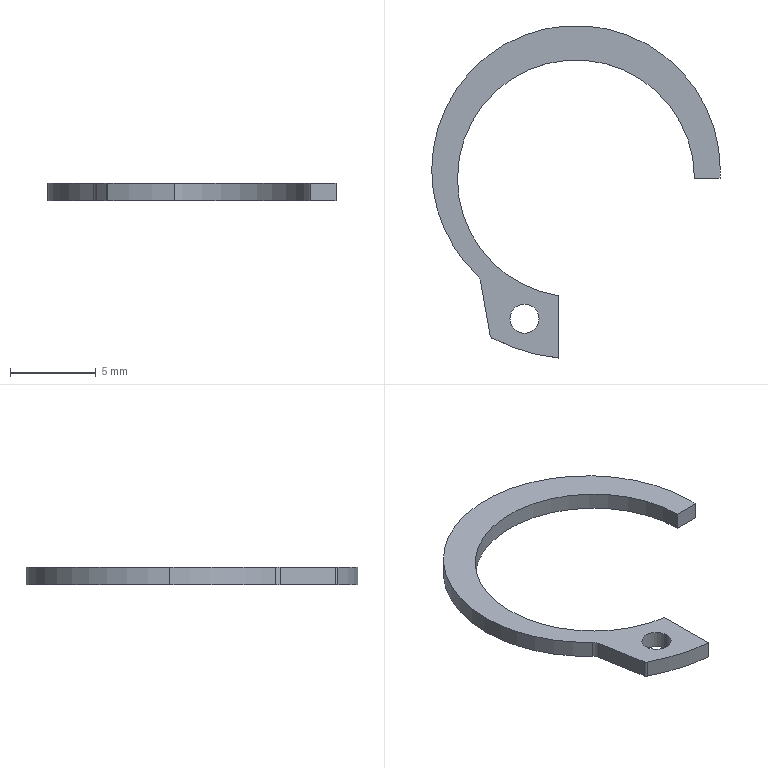Part | STEP file | Shaft retaining ring type A 15 | 1 solid | 15 faces | box 16.8 x 19.352 x 1 mm | volume 66.829 mm3 | cylinder 10 | plane 5 | commonest cylinder face diameters 16.8 x3 1.7 x2 13.8 x2 0.4 x1 1 x1 21 x1
STEP:
#1=CARTESIAN_POINT('',(0.,0.,0.));
#2=DIRECTION('',(0.,0.,1.));
#3=DIRECTION('',(1.,0.,0.));
#4=AXIS2_PLACEMENT_3D('',#1,#2,#3);
#5=CARTESIAN_POINT('',(-3.85,-8.666,0.5));
#6=VERTEX_POINT('',#5);
#7=CARTESIAN_POINT('',(-3.85,-8.666,-0.5));
#8=VERTEX_POINT('',#7);
#9=CARTESIAN_POINT('',(-3.85,-8.666,0.5));
#10=DIRECTION('',(0.,0.,-1.));
#11=VECTOR('',#10,1.);
#12=LINE('',#9,#11);
#13=CARTESIAN_POINT('',(-3.,-8.666,0.5));
#14=DIRECTION('',(0.,0.,-1.));
#15=DIRECTION('',(-1.,0.,0.));
#16=AXIS2_PLACEMENT_3D('',#13,#14,#15);
#17=CYLINDRICAL_SURFACE('',#16,0.85);
#18=CARTESIAN_POINT('',(6.283,0.));
#19=DIRECTION('',(0.,1.));
#20=VECTOR('',#19,1.);
#21=LINE('',#18,#20);
#22=(GEOMETRIC_REPRESENTATION_CONTEXT(2)PARAMETRIC_REPRESENTATION_CONTEXT()REPRESENTATION_CONTEXT('',''));
#23=DEFINITIONAL_REPRESENTATION('',(#21),#22);
#24=PCURVE('',#17,#23);
#25=CARTESIAN_POINT('',(-3.,-8.666,0.5));
#26=DIRECTION('',(0.,0.,-1.));
#27=DIRECTION('',(-1.,0.,0.));
#28=AXIS2_PLACEMENT_3D('',#25,#26,#27);
#29=CYLINDRICAL_SURFACE('',#28,0.85);
#30=CARTESIAN_POINT('',(0.,0.));
#31=DIRECTION('',(0.,1.));
#32=VECTOR('',#31,1.);
#33=LINE('',#30,#32);
#34=(GEOMETRIC_REPRESENTATION_CONTEXT(2)PARAMETRIC_REPRESENTATION_CONTEXT()REPRESENTATION_CONTEXT('',''));
#35=DEFINITIONAL_REPRESENTATION('',(#33),#34);
#36=PCURVE('',#29,#35);
#37=SURFACE_CURVE('',#12,(#24,#36),.PCURVE_S1.);
#38=EDGE_CURVE('',#6,#8,#37,.T.);
#39=ORIENTED_EDGE('',*,*,#38,.T.);
#40=CARTESIAN_POINT('',(-2.15,-8.666,-0.5));
#41=VERTEX_POINT('',#40);
#42=CARTESIAN_POINT('',(-3.,-8.666,-0.5));
#43=DIRECTION('',(0.,0.,1.));
#44=DIRECTION('',(1.,0.,0.));
#45=AXIS2_PLACEMENT_3D('',#42,#43,#44);
#46=CIRCLE('',#45,0.85);
#47=CARTESIAN_POINT('',(9.425,1.));
#48=DIRECTION('',(-1.,0.));
#49=VECTOR('',#48,1.);
#50=LINE('',#47,#49);
#51=(GEOMETRIC_REPRESENTATION_CONTEXT(2)PARAMETRIC_REPRESENTATION_CONTEXT()REPRESENTATION_CONTEXT('',''));
#52=DEFINITIONAL_REPRESENTATION('',(#50),#51);
#53=PCURVE('',#17,#52);
#54=CARTESIAN_POINT('',(-6.059,-6.519,-0.5));
#55=DIRECTION('',(0.,0.,1.));
#56=DIRECTION('',(1.,0.,0.));
#57=AXIS2_PLACEMENT_3D('',#54,#55,#56);
#58=PLANE('',#57);
#59=CARTESIAN_POINT('',(3.059,-2.147));
#60=DIRECTION('',(1.,0.));
#61=AXIS2_PLACEMENT_2D('',#59,#60);
#62=CIRCLE('',#61,0.85);
#63=(GEOMETRIC_REPRESENTATION_CONTEXT(2)PARAMETRIC_REPRESENTATION_CONTEXT()REPRESENTATION_CONTEXT('',''));
#64=DEFINITIONAL_REPRESENTATION('',(#62),#63);
#65=PCURVE('',#58,#64);
#66=SURFACE_CURVE('',#46,(#53,#65),.PCURVE_S1.);
#67=EDGE_CURVE('',#8,#41,#66,.T.);
#68=ORIENTED_EDGE('',*,*,#67,.T.);
#69=CARTESIAN_POINT('',(-2.15,-8.666,0.5));
#70=VERTEX_POINT('',#69);
#71=CARTESIAN_POINT('',(-2.15,-8.666,0.5));
#72=DIRECTION('',(0.,0.,-1.));
#73=VECTOR('',#72,1.);
#74=LINE('',#71,#73);
#75=CARTESIAN_POINT('',(3.142,0.));
#76=DIRECTION('',(0.,1.));
#77=VECTOR('',#76,1.);
#78=LINE('',#75,#77);
#79=(GEOMETRIC_REPRESENTATION_CONTEXT(2)PARAMETRIC_REPRESENTATION_CONTEXT()REPRESENTATION_CONTEXT('',''));
#80=DEFINITIONAL_REPRESENTATION('',(#78),#79);
#81=PCURVE('',#17,#80);
#82=CARTESIAN_POINT('',(3.142,0.));
#83=DIRECTION('',(0.,1.));
#84=VECTOR('',#83,1.);
#85=LINE('',#82,#84);
#86=(GEOMETRIC_REPRESENTATION_CONTEXT(2)PARAMETRIC_REPRESENTATION_CONTEXT()REPRESENTATION_CONTEXT('',''));
#87=DEFINITIONAL_REPRESENTATION('',(#85),#86);
#88=PCURVE('',#29,#87);
#89=SURFACE_CURVE('',#74,(#81,#88),.PCURVE_S1.);
#90=EDGE_CURVE('',#70,#41,#89,.T.);
#91=ORIENTED_EDGE('',*,*,#90,.F.);
#92=CARTESIAN_POINT('',(-3.,-8.666,0.5));
#93=DIRECTION('',(0.,0.,1.));
#94=DIRECTION('',(1.,0.,0.));
#95=AXIS2_PLACEMENT_3D('',#92,#93,#94);
#96=CIRCLE('',#95,0.85);
#97=CARTESIAN_POINT('',(9.425,0.));
#98=DIRECTION('',(-1.,0.));
#99=VECTOR('',#98,1.);
#100=LINE('',#97,#99);
#101=(GEOMETRIC_REPRESENTATION_CONTEXT(2)PARAMETRIC_REPRESENTATION_CONTEXT()REPRESENTATION_CONTEXT('',''));
#102=DEFINITIONAL_REPRESENTATION('',(#100),#101);
#103=PCURVE('',#17,#102);
#104=CARTESIAN_POINT('',(-6.059,-6.519,0.5));
#105=DIRECTION('',(0.,0.,1.));
#106=DIRECTION('',(1.,0.,0.));
#107=AXIS2_PLACEMENT_3D('',#104,#105,#106);
#108=PLANE('',#107);
#109=CARTESIAN_POINT('',(3.059,-2.147));
#110=DIRECTION('',(1.,0.));
#111=AXIS2_PLACEMENT_2D('',#109,#110);
#112=CIRCLE('',#111,0.85);
#113=(GEOMETRIC_REPRESENTATION_CONTEXT(2)PARAMETRIC_REPRESENTATION_CONTEXT()REPRESENTATION_CONTEXT('',''));
#114=DEFINITIONAL_REPRESENTATION('',(#112),#113);
#115=PCURVE('',#108,#114);
#116=SURFACE_CURVE('',#96,(#103,#115),.PCURVE_S1.);
#117=EDGE_CURVE('',#6,#70,#116,.T.);
#118=ORIENTED_EDGE('',*,*,#117,.F.);
#119=EDGE_LOOP('',(#39,#68,#91,#118));
#120=FACE_BOUND('',#119,.F.);
#121=ADVANCED_FACE('',(#120),#17,.F.);
#122=CARTESIAN_POINT('',(8.4,0.,0.5));
#123=VERTEX_POINT('',#122);
#124=CARTESIAN_POINT('',(-8.4,0.,0.5));
#125=VERTEX_POINT('',#124);
#126=CARTESIAN_POINT('',(0.,0.,0.5));
#127=DIRECTION('',(0.,0.,1.));
#128=DIRECTION('',(1.,0.,0.));
#129=AXIS2_PLACEMENT_3D('',#126,#127,#128);
#130=CIRCLE('',#129,8.4);
#131=CARTESIAN_POINT('',(0.,0.,0.5));
#132=DIRECTION('',(0.,0.,-1.));
#133=DIRECTION('',(-1.,0.,0.));
#134=AXIS2_PLACEMENT_3D('',#131,#132,#133);
#135=CYLINDRICAL_SURFACE('',#134,8.4);
#136=CARTESIAN_POINT('',(3.142,0.));
#137=DIRECTION('',(-1.,0.));
#138=VECTOR('',#137,1.);
#139=LINE('',#136,#138);
#140=(GEOMETRIC_REPRESENTATION_CONTEXT(2)PARAMETRIC_REPRESENTATION_CONTEXT()REPRESENTATION_CONTEXT('',''));
#141=DEFINITIONAL_REPRESENTATION('',(#139),#140);
#142=PCURVE('',#135,#141);
#143=CARTESIAN_POINT('',(6.059,6.519));
#144=DIRECTION('',(1.,0.));
#145=AXIS2_PLACEMENT_2D('',#143,#144);
#146=CIRCLE('',#145,8.4);
#147=(GEOMETRIC_REPRESENTATION_CONTEXT(2)PARAMETRIC_REPRESENTATION_CONTEXT()REPRESENTATION_CONTEXT('',''));
#148=DEFINITIONAL_REPRESENTATION('',(#146),#147);
#149=PCURVE('',#108,#148);
#150=SURFACE_CURVE('',#130,(#142,#149),.PCURVE_S1.);
#151=EDGE_CURVE('',#123,#125,#150,.T.);
#152=ORIENTED_EDGE('',*,*,#151,.F.);
#153=CARTESIAN_POINT('',(8.4,0.,-0.5));
#154=VERTEX_POINT('',#153);
#155=CARTESIAN_POINT('',(8.4,0.,0.5));
#156=DIRECTION('',(0.,0.,-1.));
#157=VECTOR('',#156,1.);
#158=LINE('',#155,#157);
#159=CARTESIAN_POINT('',(3.142,0.));
#160=DIRECTION('',(0.,1.));
#161=VECTOR('',#160,1.);
#162=LINE('',#159,#161);
#163=(GEOMETRIC_REPRESENTATION_CONTEXT(2)PARAMETRIC_REPRESENTATION_CONTEXT()REPRESENTATION_CONTEXT('',''));
#164=DEFINITIONAL_REPRESENTATION('',(#162),#163);
#165=PCURVE('',#135,#164);
#166=CARTESIAN_POINT('',(0.,0.,0.5));
#167=DIRECTION('',(0.,0.,-1.));
#168=DIRECTION('',(-1.,0.,0.));
#169=AXIS2_PLACEMENT_3D('',#166,#167,#168);
#170=CYLINDRICAL_SURFACE('',#169,8.4);
#171=CARTESIAN_POINT('',(3.142,0.));
#172=DIRECTION('',(0.,1.));
#173=VECTOR('',#172,1.);
#174=LINE('',#171,#173);
#175=(GEOMETRIC_REPRESENTATION_CONTEXT(2)PARAMETRIC_REPRESENTATION_CONTEXT()REPRESENTATION_CONTEXT('',''));
#176=DEFINITIONAL_REPRESENTATION('',(#174),#175);
#177=PCURVE('',#170,#176);
#178=SURFACE_CURVE('',#158,(#165,#177),.PCURVE_S1.);
#179=EDGE_CURVE('',#123,#154,#178,.T.);
#180=ORIENTED_EDGE('',*,*,#179,.T.);
#181=CARTESIAN_POINT('',(-8.4,0.,-0.5));
#182=VERTEX_POINT('',#181);
#183=CARTESIAN_POINT('',(0.,0.,-0.5));
#184=DIRECTION('',(0.,0.,1.));
#185=DIRECTION('',(1.,0.,0.));
#186=AXIS2_PLACEMENT_3D('',#183,#184,#185);
#187=CIRCLE('',#186,8.4);
#188=CARTESIAN_POINT('',(3.142,1.));
#189=DIRECTION('',(-1.,0.));
#190=VECTOR('',#189,1.);
#191=LINE('',#188,#190);
#192=(GEOMETRIC_REPRESENTATION_CONTEXT(2)PARAMETRIC_REPRESENTATION_CONTEXT()REPRESENTATION_CONTEXT('',''));
#193=DEFINITIONAL_REPRESENTATION('',(#191),#192);
#194=PCURVE('',#135,#193);
#195=CARTESIAN_POINT('',(6.059,6.519));
#196=DIRECTION('',(1.,0.));
#197=AXIS2_PLACEMENT_2D('',#195,#196);
#198=CIRCLE('',#197,8.4);
#199=(GEOMETRIC_REPRESENTATION_CONTEXT(2)PARAMETRIC_REPRESENTATION_CONTEXT()REPRESENTATION_CONTEXT('',''));
#200=DEFINITIONAL_REPRESENTATION('',(#198),#199);
#201=PCURVE('',#58,#200);
#202=SURFACE_CURVE('',#187,(#194,#201),.PCURVE_S1.);
#203=EDGE_CURVE('',#154,#182,#202,.T.);
#204=ORIENTED_EDGE('',*,*,#203,.T.);
#205=CARTESIAN_POINT('',(-8.4,0.,0.5));
#206=DIRECTION('',(0.,0.,-1.));
#207=VECTOR('',#206,1.);
#208=LINE('',#205,#207);
#209=CARTESIAN_POINT('',(0.,0.));
#210=DIRECTION('',(0.,1.));
#211=VECTOR('',#210,1.);
#212=LINE('',#209,#211);
#213=(GEOMETRIC_REPRESENTATION_CONTEXT(2)PARAMETRIC_REPRESENTATION_CONTEXT()REPRESENTATION_CONTEXT('',''));
#214=DEFINITIONAL_REPRESENTATION('',(#212),#213);
#215=PCURVE('',#135,#214);
#216=CARTESIAN_POINT('',(0.,0.,0.5));
#217=DIRECTION('',(0.,0.,-1.));
#218=DIRECTION('',(-1.,0.,0.));
#219=AXIS2_PLACEMENT_3D('',#216,#217,#218);
#220=CYLINDRICAL_SURFACE('',#219,8.4);
#221=CARTESIAN_POINT('',(6.283,0.));
#222=DIRECTION('',(0.,1.));
#223=VECTOR('',#222,1.);
#224=LINE('',#221,#223);
#225=(GEOMETRIC_REPRESENTATION_CONTEXT(2)PARAMETRIC_REPRESENTATION_CONTEXT()REPRESENTATION_CONTEXT('',''));
#226=DEFINITIONAL_REPRESENTATION('',(#224),#225);
#227=PCURVE('',#220,#226);
#228=SURFACE_CURVE('',#208,(#215,#227),.PCURVE_S1.);
#229=EDGE_CURVE('',#125,#182,#228,.T.);
#230=ORIENTED_EDGE('',*,*,#229,.F.);
#231=EDGE_LOOP('',(#152,#180,#204,#230));
#232=FACE_BOUND('',#231,.T.);
#233=ADVANCED_FACE('',(#232),#135,.T.);
#234=CARTESIAN_POINT('',(-5.719,-6.153,0.5));
#235=VERTEX_POINT('',#234);
#236=CARTESIAN_POINT('',(0.,0.,0.5));
#237=DIRECTION('',(0.,0.,1.));
#238=DIRECTION('',(1.,0.,0.));
#239=AXIS2_PLACEMENT_3D('',#236,#237,#238);
#240=CIRCLE('',#239,8.4);
#241=CARTESIAN_POINT('',(9.425,0.));
#242=DIRECTION('',(-1.,0.));
#243=VECTOR('',#242,1.);
#244=LINE('',#241,#243);
#245=(GEOMETRIC_REPRESENTATION_CONTEXT(2)PARAMETRIC_REPRESENTATION_CONTEXT()REPRESENTATION_CONTEXT('',''));
#246=DEFINITIONAL_REPRESENTATION('',(#244),#245);
#247=PCURVE('',#220,#246);
#248=CARTESIAN_POINT('',(6.059,6.519));
#249=DIRECTION('',(1.,0.));
#250=AXIS2_PLACEMENT_2D('',#248,#249);
#251=CIRCLE('',#250,8.4);
#252=(GEOMETRIC_REPRESENTATION_CONTEXT(2)PARAMETRIC_REPRESENTATION_CONTEXT()REPRESENTATION_CONTEXT('',''));
#253=DEFINITIONAL_REPRESENTATION('',(#251),#252);
#254=PCURVE('',#108,#253);
#255=SURFACE_CURVE('',#240,(#247,#254),.PCURVE_S1.);
#256=EDGE_CURVE('',#125,#235,#255,.T.);
#257=ORIENTED_EDGE('',*,*,#256,.F.);
#258=ORIENTED_EDGE('',*,*,#229,.T.);
#259=CARTESIAN_POINT('',(-5.719,-6.153,-0.5));
#260=VERTEX_POINT('',#259);
#261=CARTESIAN_POINT('',(0.,0.,-0.5));
#262=DIRECTION('',(0.,0.,1.));
#263=DIRECTION('',(1.,0.,0.));
#264=AXIS2_PLACEMENT_3D('',#261,#262,#263);
#265=CIRCLE('',#264,8.4);
#266=CARTESIAN_POINT('',(9.425,1.));
#267=DIRECTION('',(-1.,0.));
#268=VECTOR('',#267,1.);
#269=LINE('',#266,#268);
#270=(GEOMETRIC_REPRESENTATION_CONTEXT(2)PARAMETRIC_REPRESENTATION_CONTEXT()REPRESENTATION_CONTEXT('',''));
#271=DEFINITIONAL_REPRESENTATION('',(#269),#270);
#272=PCURVE('',#220,#271);
#273=CARTESIAN_POINT('',(6.059,6.519));
#274=DIRECTION('',(1.,0.));
#275=AXIS2_PLACEMENT_2D('',#273,#274);
#276=CIRCLE('',#275,8.4);
#277=(GEOMETRIC_REPRESENTATION_CONTEXT(2)PARAMETRIC_REPRESENTATION_CONTEXT()REPRESENTATION_CONTEXT('',''));
#278=DEFINITIONAL_REPRESENTATION('',(#276),#277);
#279=PCURVE('',#58,#278);
#280=SURFACE_CURVE('',#265,(#272,#279),.PCURVE_S1.);
#281=EDGE_CURVE('',#182,#260,#280,.T.);
#282=ORIENTED_EDGE('',*,*,#281,.T.);
#283=CARTESIAN_POINT('',(-5.719,-6.153,0.5));
#284=DIRECTION('',(0.,0.,-1.));
#285=VECTOR('',#284,1.);
#286=LINE('',#283,#285);
#287=CARTESIAN_POINT('',(5.461,0.));
#288=DIRECTION('',(0.,1.));
#289=VECTOR('',#288,1.);
#290=LINE('',#287,#289);
#291=(GEOMETRIC_REPRESENTATION_CONTEXT(2)PARAMETRIC_REPRESENTATION_CONTEXT()REPRESENTATION_CONTEXT('',''));
#292=DEFINITIONAL_REPRESENTATION('',(#290),#291);
#293=PCURVE('',#220,#292);
#294=CARTESIAN_POINT('',(-6.059,-6.519,0.5));
#295=DIRECTION('',(0.,0.,-1.));
#296=DIRECTION('',(-1.,0.,0.));
#297=AXIS2_PLACEMENT_3D('',#294,#295,#296);
#298=CYLINDRICAL_SURFACE('',#297,0.5);
#299=CARTESIAN_POINT('',(2.32,0.));
#300=DIRECTION('',(0.,1.));
#301=VECTOR('',#300,1.);
#302=LINE('',#299,#301);
#303=(GEOMETRIC_REPRESENTATION_CONTEXT(2)PARAMETRIC_REPRESENTATION_CONTEXT()REPRESENTATION_CONTEXT('',''));
#304=DEFINITIONAL_REPRESENTATION('',(#302),#303);
#305=PCURVE('',#298,#304);
#306=SURFACE_CURVE('',#286,(#293,#305),.PCURVE_S1.);
#307=EDGE_CURVE('',#235,#260,#306,.T.);
#308=ORIENTED_EDGE('',*,*,#307,.F.);
#309=EDGE_LOOP('',(#257,#258,#282,#308));
#310=FACE_BOUND('',#309,.T.);
#311=ADVANCED_FACE('',(#310),#220,.T.);
#312=CARTESIAN_POINT('',(6.9,-0.5,-0.5));
#313=VERTEX_POINT('',#312);
#314=CARTESIAN_POINT('',(6.9,-0.5,0.5));
#315=VERTEX_POINT('',#314);
#316=CARTESIAN_POINT('',(6.9,-0.5,0.5));
#317=DIRECTION('',(0.,0.,1.));
#318=VECTOR('',#317,1.);
#319=LINE('',#316,#318);
#320=CARTESIAN_POINT('',(0.,-0.5,0.5));
#321=DIRECTION('',(0.,0.,-1.));
#322=DIRECTION('',(-1.,0.,0.));
#323=AXIS2_PLACEMENT_3D('',#320,#321,#322);
#324=CYLINDRICAL_SURFACE('',#323,6.9);
#325=CARTESIAN_POINT('',(3.142,0.));
#326=DIRECTION('',(0.,-1.));
#327=VECTOR('',#326,1.);
#328=LINE('',#325,#327);
#329=(GEOMETRIC_REPRESENTATION_CONTEXT(2)PARAMETRIC_REPRESENTATION_CONTEXT()REPRESENTATION_CONTEXT('',''));
#330=DEFINITIONAL_REPRESENTATION('',(#328),#329);
#331=PCURVE('',#324,#330);
#332=CARTESIAN_POINT('',(0.,-0.5,-37.5));
#333=DIRECTION('',(0.,1.,0.));
#334=DIRECTION('',(-1.,0.,0.));
#335=AXIS2_PLACEMENT_3D('',#332,#333,#334);
#336=PLANE('',#335);
#337=CARTESIAN_POINT('',(-6.9,38.));
#338=DIRECTION('',(0.,1.));
#339=VECTOR('',#338,1.);
#340=LINE('',#337,#339);
#341=(GEOMETRIC_REPRESENTATION_CONTEXT(2)PARAMETRIC_REPRESENTATION_CONTEXT()REPRESENTATION_CONTEXT('',''));
#342=DEFINITIONAL_REPRESENTATION('',(#340),#341);
#343=PCURVE('',#336,#342);
#344=SURFACE_CURVE('',#319,(#331,#343),.PCURVE_S1.);
#345=EDGE_CURVE('',#313,#315,#344,.T.);
#346=ORIENTED_EDGE('',*,*,#345,.F.);
#347=CARTESIAN_POINT('',(-6.9,-0.5,-0.5));
#348=VERTEX_POINT('',#347);
#349=CARTESIAN_POINT('',(0.,-0.5,-0.5));
#350=DIRECTION('',(0.,0.,-1.));
#351=DIRECTION('',(1.,0.,0.));
#352=AXIS2_PLACEMENT_3D('',#349,#350,#351);
#353=CIRCLE('',#352,6.9);
#354=CARTESIAN_POINT('',(-3.142,1.));
#355=DIRECTION('',(1.,0.));
#356=VECTOR('',#355,1.);
#357=LINE('',#354,#356);
#358=(GEOMETRIC_REPRESENTATION_CONTEXT(2)PARAMETRIC_REPRESENTATION_CONTEXT()REPRESENTATION_CONTEXT('',''));
#359=DEFINITIONAL_REPRESENTATION('',(#357),#358);
#360=PCURVE('',#324,#359);
#361=CARTESIAN_POINT('',(12.959,6.019));
#362=CARTESIAN_POINT('',(12.959,-5.932));
#363=CARTESIAN_POINT('',(2.609,0.04337));
#364=CARTESIAN_POINT('',(-7.741,6.019));
#365=CARTESIAN_POINT('',(2.609,11.995));
#366=CARTESIAN_POINT('',(12.959,17.97));
#367=CARTESIAN_POINT('',(12.959,6.019));
#368=(BOUNDED_CURVE()B_SPLINE_CURVE(2,(#361,#362,#363,#364,#365,#366,#367),.UNSPECIFIED.,.T.,.F.)B_SPLINE_CURVE_WITH_KNOTS((1,2,2,2,2,1),(-2.094,0.,2.094,4.189,6.283,8.378),.UNSPECIFIED.)CURVE()GEOMETRIC_REPRESENTATION_ITEM()RATIONAL_B_SPLINE_CURVE((1.,0.5,1.,0.5,1.,0.5,1.))REPRESENTATION_ITEM(''));
#369=(GEOMETRIC_REPRESENTATION_CONTEXT(2)PARAMETRIC_REPRESENTATION_CONTEXT()REPRESENTATION_CONTEXT('',''));
#370=DEFINITIONAL_REPRESENTATION('',(#368),#369);
#371=PCURVE('',#58,#370);
#372=SURFACE_CURVE('',#353,(#360,#371),.PCURVE_S1.);
#373=EDGE_CURVE('',#348,#313,#372,.T.);
#374=ORIENTED_EDGE('',*,*,#373,.F.);
#375=CARTESIAN_POINT('',(-6.9,-0.5,0.5));
#376=VERTEX_POINT('',#375);
#377=CARTESIAN_POINT('',(-6.9,-0.5,0.5));
#378=DIRECTION('',(0.,0.,-1.));
#379=VECTOR('',#378,1.);
#380=LINE('',#377,#379);
#381=CARTESIAN_POINT('',(0.,0.));
#382=DIRECTION('',(0.,1.));
#383=VECTOR('',#382,1.);
#384=LINE('',#381,#383);
#385=(GEOMETRIC_REPRESENTATION_CONTEXT(2)PARAMETRIC_REPRESENTATION_CONTEXT()REPRESENTATION_CONTEXT('',''));
#386=DEFINITIONAL_REPRESENTATION('',(#384),#385);
#387=PCURVE('',#324,#386);
#388=CARTESIAN_POINT('',(0.,-0.5,0.5));
#389=DIRECTION('',(0.,0.,-1.));
#390=DIRECTION('',(-1.,0.,0.));
#391=AXIS2_PLACEMENT_3D('',#388,#389,#390);
#392=CYLINDRICAL_SURFACE('',#391,6.9);
#393=CARTESIAN_POINT('',(6.283,0.));
#394=DIRECTION('',(0.,1.));
#395=VECTOR('',#394,1.);
#396=LINE('',#393,#395);
#397=(GEOMETRIC_REPRESENTATION_CONTEXT(2)PARAMETRIC_REPRESENTATION_CONTEXT()REPRESENTATION_CONTEXT('',''));
#398=DEFINITIONAL_REPRESENTATION('',(#396),#397);
#399=PCURVE('',#392,#398);
#400=SURFACE_CURVE('',#380,(#387,#399),.PCURVE_S1.);
#401=EDGE_CURVE('',#376,#348,#400,.T.);
#402=ORIENTED_EDGE('',*,*,#401,.F.);
#403=CARTESIAN_POINT('',(0.,-0.5,0.5));
#404=DIRECTION('',(0.,0.,-1.));
#405=DIRECTION('',(1.,0.,0.));
#406=AXIS2_PLACEMENT_3D('',#403,#404,#405);
#407=CIRCLE('',#406,6.9);
#408=CARTESIAN_POINT('',(-3.142,0.));
#409=DIRECTION('',(1.,0.));
#410=VECTOR('',#409,1.);
#411=LINE('',#408,#410);
#412=(GEOMETRIC_REPRESENTATION_CONTEXT(2)PARAMETRIC_REPRESENTATION_CONTEXT()REPRESENTATION_CONTEXT('',''));
#413=DEFINITIONAL_REPRESENTATION('',(#411),#412);
#414=PCURVE('',#324,#413);
#415=CARTESIAN_POINT('',(12.959,6.019));
#416=CARTESIAN_POINT('',(12.959,-5.932));
#417=CARTESIAN_POINT('',(2.609,0.04337));
#418=CARTESIAN_POINT('',(-7.741,6.019));
#419=CARTESIAN_POINT('',(2.609,11.995));
#420=CARTESIAN_POINT('',(12.959,17.97));
#421=CARTESIAN_POINT('',(12.959,6.019));
#422=(BOUNDED_CURVE()B_SPLINE_CURVE(2,(#415,#416,#417,#418,#419,#420,#421),.UNSPECIFIED.,.T.,.F.)B_SPLINE_CURVE_WITH_KNOTS((1,2,2,2,2,1),(-2.094,0.,2.094,4.189,6.283,8.378),.UNSPECIFIED.)CURVE()GEOMETRIC_REPRESENTATION_ITEM()RATIONAL_B_SPLINE_CURVE((1.,0.5,1.,0.5,1.,0.5,1.))REPRESENTATION_ITEM(''));
#423=(GEOMETRIC_REPRESENTATION_CONTEXT(2)PARAMETRIC_REPRESENTATION_CONTEXT()REPRESENTATION_CONTEXT('',''));
#424=DEFINITIONAL_REPRESENTATION('',(#422),#423);
#425=PCURVE('',#108,#424);
#426=SURFACE_CURVE('',#407,(#414,#425),.PCURVE_S1.);
#427=EDGE_CURVE('',#376,#315,#426,.T.);
#428=ORIENTED_EDGE('',*,*,#427,.T.);
#429=EDGE_LOOP('',(#346,#374,#402,#428));
#430=FACE_BOUND('',#429,.F.);
#431=ADVANCED_FACE('',(#430),#324,.F.);
#432=CARTESIAN_POINT('',(8.385,-0.5,0.5));
#433=VERTEX_POINT('',#432);
#434=CARTESIAN_POINT('',(-6.059,-0.5,0.5));
#435=DIRECTION('',(-1.,0.,0.));
#436=VECTOR('',#435,1.);
#437=LINE('',#434,#436);
#438=CARTESIAN_POINT('',(0.,6.019));
#439=DIRECTION('',(-1.,0.));
#440=VECTOR('',#439,1.);
#441=LINE('',#438,#440);
#442=(GEOMETRIC_REPRESENTATION_CONTEXT(2)PARAMETRIC_REPRESENTATION_CONTEXT()REPRESENTATION_CONTEXT('',''));
#443=DEFINITIONAL_REPRESENTATION('',(#441),#442);
#444=PCURVE('',#108,#443);
#445=CARTESIAN_POINT('',(6.059,38.));
#446=DIRECTION('',(1.,0.));
#447=VECTOR('',#446,1.);
#448=LINE('',#445,#447);
#449=(GEOMETRIC_REPRESENTATION_CONTEXT(2)PARAMETRIC_REPRESENTATION_CONTEXT()REPRESENTATION_CONTEXT('',''));
#450=DEFINITIONAL_REPRESENTATION('',(#448),#449);
#451=PCURVE('',#336,#450);
#452=SURFACE_CURVE('',#437,(#444,#451),.PCURVE_S1.);
#453=EDGE_CURVE('',#433,#315,#452,.T.);
#454=ORIENTED_EDGE('',*,*,#453,.F.);
#455=CARTESIAN_POINT('',(0.,0.,0.5));
#456=DIRECTION('',(0.,0.,1.));
#457=DIRECTION('',(1.,0.,0.));
#458=AXIS2_PLACEMENT_3D('',#455,#456,#457);
#459=CIRCLE('',#458,8.4);
#460=CARTESIAN_POINT('',(6.059,6.519));
#461=DIRECTION('',(1.,0.));
#462=AXIS2_PLACEMENT_2D('',#460,#461);
#463=CIRCLE('',#462,8.4);
#464=(GEOMETRIC_REPRESENTATION_CONTEXT(2)PARAMETRIC_REPRESENTATION_CONTEXT()REPRESENTATION_CONTEXT('',''));
#465=DEFINITIONAL_REPRESENTATION('',(#463),#464);
#466=PCURVE('',#108,#465);
#467=CARTESIAN_POINT('',(9.425,0.));
#468=DIRECTION('',(-1.,0.));
#469=VECTOR('',#468,1.);
#470=LINE('',#467,#469);
#471=(GEOMETRIC_REPRESENTATION_CONTEXT(2)PARAMETRIC_REPRESENTATION_CONTEXT()REPRESENTATION_CONTEXT('',''));
#472=DEFINITIONAL_REPRESENTATION('',(#470),#471);
#473=PCURVE('',#170,#472);
#474=SURFACE_CURVE('',#459,(#466,#473),.PCURVE_S1.);
#475=EDGE_CURVE('',#433,#123,#474,.T.);
#476=ORIENTED_EDGE('',*,*,#475,.T.);
#477=ORIENTED_EDGE('',*,*,#151,.T.);
#478=ORIENTED_EDGE('',*,*,#256,.T.);
#479=CARTESIAN_POINT('',(-5.567,-6.432,0.5));
#480=VERTEX_POINT('',#479);
#481=CARTESIAN_POINT('',(-6.059,-6.519,0.5));
#482=DIRECTION('',(0.,0.,-1.));
#483=DIRECTION('',(1.,0.,0.));
#484=AXIS2_PLACEMENT_3D('',#481,#482,#483);
#485=CIRCLE('',#484,0.5);
#486=CARTESIAN_POINT('',(0.5,0.));
#487=CARTESIAN_POINT('',(0.5,-0.866));
#488=CARTESIAN_POINT('',(-0.25,-0.433));
#489=CARTESIAN_POINT('',(-1.,0.));
#490=CARTESIAN_POINT('',(-0.25,0.433));
#491=CARTESIAN_POINT('',(0.5,0.866));
#492=CARTESIAN_POINT('',(0.5,0.));
#493=(BOUNDED_CURVE()B_SPLINE_CURVE(2,(#486,#487,#488,#489,#490,#491,#492),.UNSPECIFIED.,.T.,.F.)B_SPLINE_CURVE_WITH_KNOTS((1,2,2,2,2,1),(-2.094,0.,2.094,4.189,6.283,8.378),.UNSPECIFIED.)CURVE()GEOMETRIC_REPRESENTATION_ITEM()RATIONAL_B_SPLINE_CURVE((1.,0.5,1.,0.5,1.,0.5,1.))REPRESENTATION_ITEM(''));
#494=(GEOMETRIC_REPRESENTATION_CONTEXT(2)PARAMETRIC_REPRESENTATION_CONTEXT()REPRESENTATION_CONTEXT('',''));
#495=DEFINITIONAL_REPRESENTATION('',(#493),#494);
#496=PCURVE('',#108,#495);
#497=CARTESIAN_POINT('',(-3.142,0.));
#498=DIRECTION('',(1.,0.));
#499=VECTOR('',#498,1.);
#500=LINE('',#497,#499);
#501=(GEOMETRIC_REPRESENTATION_CONTEXT(2)PARAMETRIC_REPRESENTATION_CONTEXT()REPRESENTATION_CONTEXT('',''));
#502=DEFINITIONAL_REPRESENTATION('',(#500),#501);
#503=PCURVE('',#298,#502);
#504=SURFACE_CURVE('',#485,(#496,#503),.PCURVE_S1.);
#505=EDGE_CURVE('',#235,#480,#504,.T.);
#506=ORIENTED_EDGE('',*,*,#505,.T.);
#507=CARTESIAN_POINT('',(-5.,-9.646,0.5));
#508=VERTEX_POINT('',#507);
#509=CARTESIAN_POINT('',(-5.567,-6.432,0.5));
#510=DIRECTION('',(0.1736,-0.9848,0.));
#511=VECTOR('',#510,1.);
#512=LINE('',#509,#511);
#513=CARTESIAN_POINT('',(0.4924,0.08682));
#514=DIRECTION('',(0.1736,-0.9848));
#515=VECTOR('',#514,1.);
#516=LINE('',#513,#515);
#517=(GEOMETRIC_REPRESENTATION_CONTEXT(2)PARAMETRIC_REPRESENTATION_CONTEXT()REPRESENTATION_CONTEXT('',''));
#518=DEFINITIONAL_REPRESENTATION('',(#516),#517);
#519=PCURVE('',#108,#518);
#520=CARTESIAN_POINT('',(-5.567,-6.432,0.5));
#521=DIRECTION('',(0.9848,0.1736,0.));
#522=DIRECTION('',(-0.1736,0.9848,0.));
#523=AXIS2_PLACEMENT_3D('',#520,#521,#522);
#524=PLANE('',#523);
#525=CARTESIAN_POINT('',(0.,0.));
#526=DIRECTION('',(-1.,0.));
#527=VECTOR('',#526,1.);
#528=LINE('',#525,#527);
#529=(GEOMETRIC_REPRESENTATION_CONTEXT(2)PARAMETRIC_REPRESENTATION_CONTEXT()REPRESENTATION_CONTEXT('',''));
#530=DEFINITIONAL_REPRESENTATION('',(#528),#529);
#531=PCURVE('',#524,#530);
#532=SURFACE_CURVE('',#512,(#519,#531),.PCURVE_S1.);
#533=EDGE_CURVE('',#480,#508,#532,.T.);
#534=ORIENTED_EDGE('',*,*,#533,.T.);
#535=CARTESIAN_POINT('',(-4.896,-9.789,0.5));
#536=VERTEX_POINT('',#535);
#537=CARTESIAN_POINT('',(-4.803,-9.612,0.5));
#538=DIRECTION('',(0.,0.,1.));
#539=DIRECTION('',(-1.,0.,0.));
#540=AXIS2_PLACEMENT_3D('',#537,#538,#539);
#541=CIRCLE('',#540,0.2);
#542=CARTESIAN_POINT('',(1.256,-3.093));
#543=DIRECTION('',(-1.,0.));
#544=AXIS2_PLACEMENT_2D('',#542,#543);
#545=CIRCLE('',#544,0.2);
#546=(GEOMETRIC_REPRESENTATION_CONTEXT(2)PARAMETRIC_REPRESENTATION_CONTEXT()REPRESENTATION_CONTEXT('',''));
#547=DEFINITIONAL_REPRESENTATION('',(#545),#546);
#548=PCURVE('',#108,#547);
#549=CARTESIAN_POINT('',(-4.803,-9.612,0.5));
#550=DIRECTION('',(0.,0.,-1.));
#551=DIRECTION('',(-1.,0.,0.));
#552=AXIS2_PLACEMENT_3D('',#549,#550,#551);
#553=CYLINDRICAL_SURFACE('',#552,0.2);
#554=CARTESIAN_POINT('',(6.283,0.));
#555=DIRECTION('',(-1.,0.));
#556=VECTOR('',#555,1.);
#557=LINE('',#554,#556);
#558=(GEOMETRIC_REPRESENTATION_CONTEXT(2)PARAMETRIC_REPRESENTATION_CONTEXT()REPRESENTATION_CONTEXT('',''));
#559=DEFINITIONAL_REPRESENTATION('',(#557),#558);
#560=PCURVE('',#553,#559);
#561=SURFACE_CURVE('',#541,(#548,#560),.PCURVE_S1.);
#562=EDGE_CURVE('',#508,#536,#561,.T.);
#563=ORIENTED_EDGE('',*,*,#562,.T.);
#564=CARTESIAN_POINT('',(-1.,-10.952,0.5));
#565=VERTEX_POINT('',#564);
#566=CARTESIAN_POINT('',(0.,-0.5,0.5));
#567=DIRECTION('',(0.,0.,1.));
#568=DIRECTION('',(-1.,0.,0.));
#569=AXIS2_PLACEMENT_3D('',#566,#567,#568);
#570=CIRCLE('',#569,10.5);
#571=CARTESIAN_POINT('',(6.059,6.019));
#572=DIRECTION('',(-1.,0.));
#573=AXIS2_PLACEMENT_2D('',#571,#572);
#574=CIRCLE('',#573,10.5);
#575=(GEOMETRIC_REPRESENTATION_CONTEXT(2)PARAMETRIC_REPRESENTATION_CONTEXT()REPRESENTATION_CONTEXT('',''));
#576=DEFINITIONAL_REPRESENTATION('',(#574),#575);
#577=PCURVE('',#108,#576);
#578=CARTESIAN_POINT('',(0.,-0.5,0.5));
#579=DIRECTION('',(0.,0.,-1.));
#580=DIRECTION('',(-1.,0.,0.));
#581=AXIS2_PLACEMENT_3D('',#578,#579,#580);
#582=CYLINDRICAL_SURFACE('',#581,10.5);
#583=CARTESIAN_POINT('',(6.283,0.));
#584=DIRECTION('',(-1.,0.));
#585=VECTOR('',#584,1.);
#586=LINE('',#583,#585);
#587=(GEOMETRIC_REPRESENTATION_CONTEXT(2)PARAMETRIC_REPRESENTATION_CONTEXT()REPRESENTATION_CONTEXT('',''));
#588=DEFINITIONAL_REPRESENTATION('',(#586),#587);
#589=PCURVE('',#582,#588);
#590=SURFACE_CURVE('',#570,(#577,#589),.PCURVE_S1.);
#591=EDGE_CURVE('',#536,#565,#590,.T.);
#592=ORIENTED_EDGE('',*,*,#591,.T.);
#593=CARTESIAN_POINT('',(-1.,-7.327,0.5));
#594=VERTEX_POINT('',#593);
#595=CARTESIAN_POINT('',(-1.,-7.327,0.5));
#596=DIRECTION('',(0.,1.,0.));
#597=VECTOR('',#596,1.);
#598=LINE('',#595,#597);
#599=CARTESIAN_POINT('',(5.059,-0.8082));
#600=DIRECTION('',(0.,1.));
#601=VECTOR('',#600,1.);
#602=LINE('',#599,#601);
#603=(GEOMETRIC_REPRESENTATION_CONTEXT(2)PARAMETRIC_REPRESENTATION_CONTEXT()REPRESENTATION_CONTEXT('',''));
#604=DEFINITIONAL_REPRESENTATION('',(#602),#603);
#605=PCURVE('',#108,#604);
#606=CARTESIAN_POINT('',(-1.,-7.327,0.5));
#607=DIRECTION('',(-1.,0.,0.));
#608=DIRECTION('',(0.,-1.,0.));
#609=AXIS2_PLACEMENT_3D('',#606,#607,#608);
#610=PLANE('',#609);
#611=CARTESIAN_POINT('',(0.,0.));
#612=DIRECTION('',(-1.,0.));
#613=VECTOR('',#612,1.);
#614=LINE('',#611,#613);
#615=(GEOMETRIC_REPRESENTATION_CONTEXT(2)PARAMETRIC_REPRESENTATION_CONTEXT()REPRESENTATION_CONTEXT('',''));
#616=DEFINITIONAL_REPRESENTATION('',(#614),#615);
#617=PCURVE('',#610,#616);
#618=SURFACE_CURVE('',#598,(#605,#617),.PCURVE_S1.);
#619=EDGE_CURVE('',#565,#594,#618,.T.);
#620=ORIENTED_EDGE('',*,*,#619,.T.);
#621=CARTESIAN_POINT('',(0.,-0.5,0.5));
#622=DIRECTION('',(0.,0.,-1.));
#623=DIRECTION('',(1.,0.,0.));
#624=AXIS2_PLACEMENT_3D('',#621,#622,#623);
#625=CIRCLE('',#624,6.9);
#626=CARTESIAN_POINT('',(12.959,6.019));
#627=CARTESIAN_POINT('',(12.959,-5.932));
#628=CARTESIAN_POINT('',(2.609,0.04337));
#629=CARTESIAN_POINT('',(-7.741,6.019));
#630=CARTESIAN_POINT('',(2.609,11.995));
#631=CARTESIAN_POINT('',(12.959,17.97));
#632=CARTESIAN_POINT('',(12.959,6.019));
#633=(BOUNDED_CURVE()B_SPLINE_CURVE(2,(#626,#627,#628,#629,#630,#631,#632),.UNSPECIFIED.,.T.,.F.)B_SPLINE_CURVE_WITH_KNOTS((1,2,2,2,2,1),(-2.094,0.,2.094,4.189,6.283,8.378),.UNSPECIFIED.)CURVE()GEOMETRIC_REPRESENTATION_ITEM()RATIONAL_B_SPLINE_CURVE((1.,0.5,1.,0.5,1.,0.5,1.))REPRESENTATION_ITEM(''));
#634=(GEOMETRIC_REPRESENTATION_CONTEXT(2)PARAMETRIC_REPRESENTATION_CONTEXT()REPRESENTATION_CONTEXT('',''));
#635=DEFINITIONAL_REPRESENTATION('',(#633),#634);
#636=PCURVE('',#108,#635);
#637=CARTESIAN_POINT('',(3.142,0.));
#638=DIRECTION('',(1.,0.));
#639=VECTOR('',#638,1.);
#640=LINE('',#637,#639);
#641=(GEOMETRIC_REPRESENTATION_CONTEXT(2)PARAMETRIC_REPRESENTATION_CONTEXT()REPRESENTATION_CONTEXT('',''));
#642=DEFINITIONAL_REPRESENTATION('',(#640),#641);
#643=PCURVE('',#392,#642);
#644=SURFACE_CURVE('',#625,(#636,#643),.PCURVE_S1.);
#645=EDGE_CURVE('',#594,#376,#644,.T.);
#646=ORIENTED_EDGE('',*,*,#645,.T.);
#647=ORIENTED_EDGE('',*,*,#427,.T.);
#648=EDGE_LOOP('',(#454,#476,#477,#478,#506,#534,#563,#592,#620,#646,#647));
#649=FACE_BOUND('',#648,.T.);
#650=ORIENTED_EDGE('',*,*,#117,.F.);
#651=CARTESIAN_POINT('',(-3.,-8.666,0.5));
#652=DIRECTION('',(0.,0.,1.));
#653=DIRECTION('',(1.,0.,0.));
#654=AXIS2_PLACEMENT_3D('',#651,#652,#653);
#655=CIRCLE('',#654,0.85);
#656=CARTESIAN_POINT('',(3.059,-2.147));
#657=DIRECTION('',(1.,0.));
#658=AXIS2_PLACEMENT_2D('',#656,#657);
#659=CIRCLE('',#658,0.85);
#660=(GEOMETRIC_REPRESENTATION_CONTEXT(2)PARAMETRIC_REPRESENTATION_CONTEXT()REPRESENTATION_CONTEXT('',''));
#661=DEFINITIONAL_REPRESENTATION('',(#659),#660);
#662=PCURVE('',#108,#661);
#663=CARTESIAN_POINT('',(3.142,0.));
#664=DIRECTION('',(-1.,0.));
#665=VECTOR('',#664,1.);
#666=LINE('',#663,#665);
#667=(GEOMETRIC_REPRESENTATION_CONTEXT(2)PARAMETRIC_REPRESENTATION_CONTEXT()REPRESENTATION_CONTEXT('',''));
#668=DEFINITIONAL_REPRESENTATION('',(#666),#667);
#669=PCURVE('',#29,#668);
#670=SURFACE_CURVE('',#655,(#662,#669),.PCURVE_S1.);
#671=EDGE_CURVE('',#70,#6,#670,.T.);
#672=ORIENTED_EDGE('',*,*,#671,.F.);
#673=EDGE_LOOP('',(#650,#672));
#674=FACE_BOUND('',#673,.T.);
#675=ADVANCED_FACE('',(#649,#674),#108,.T.);
#676=ORIENTED_EDGE('',*,*,#505,.T.);
#677=CARTESIAN_POINT('',(-5.567,-6.432,-0.5));
#678=VERTEX_POINT('',#677);
#679=CARTESIAN_POINT('',(-5.567,-6.432,0.5));
#680=DIRECTION('',(0.,0.,-1.));
#681=VECTOR('',#680,1.);
#682=LINE('',#679,#681);
#683=CARTESIAN_POINT('',(2.967,0.));
#684=DIRECTION('',(0.,1.));
#685=VECTOR('',#684,1.);
#686=LINE('',#683,#685);
#687=(GEOMETRIC_REPRESENTATION_CONTEXT(2)PARAMETRIC_REPRESENTATION_CONTEXT()REPRESENTATION_CONTEXT('',''));
#688=DEFINITIONAL_REPRESENTATION('',(#686),#687);
#689=PCURVE('',#298,#688);
#690=CARTESIAN_POINT('',(0.,0.));
#691=DIRECTION('',(0.,-1.));
#692=VECTOR('',#691,1.);
#693=LINE('',#690,#692);
#694=(GEOMETRIC_REPRESENTATION_CONTEXT(2)PARAMETRIC_REPRESENTATION_CONTEXT()REPRESENTATION_CONTEXT('',''));
#695=DEFINITIONAL_REPRESENTATION('',(#693),#694);
#696=PCURVE('',#524,#695);
#697=SURFACE_CURVE('',#682,(#689,#696),.PCURVE_S1.);
#698=EDGE_CURVE('',#480,#678,#697,.T.);
#699=ORIENTED_EDGE('',*,*,#698,.T.);
#700=CARTESIAN_POINT('',(-6.059,-6.519,-0.5));
#701=DIRECTION('',(0.,0.,-1.));
#702=DIRECTION('',(1.,0.,0.));
#703=AXIS2_PLACEMENT_3D('',#700,#701,#702);
#704=CIRCLE('',#703,0.5);
#705=CARTESIAN_POINT('',(-3.142,1.));
#706=DIRECTION('',(1.,0.));
#707=VECTOR('',#706,1.);
#708=LINE('',#705,#707);
#709=(GEOMETRIC_REPRESENTATION_CONTEXT(2)PARAMETRIC_REPRESENTATION_CONTEXT()REPRESENTATION_CONTEXT('',''));
#710=DEFINITIONAL_REPRESENTATION('',(#708),#709);
#711=PCURVE('',#298,#710);
#712=CARTESIAN_POINT('',(0.5,0.));
#713=CARTESIAN_POINT('',(0.5,-0.866));
#714=CARTESIAN_POINT('',(-0.25,-0.433));
#715=CARTESIAN_POINT('',(-1.,0.));
#716=CARTESIAN_POINT('',(-0.25,0.433));
#717=CARTESIAN_POINT('',(0.5,0.866));
#718=CARTESIAN_POINT('',(0.5,0.));
#719=(BOUNDED_CURVE()B_SPLINE_CURVE(2,(#712,#713,#714,#715,#716,#717,#718),.UNSPECIFIED.,.T.,.F.)B_SPLINE_CURVE_WITH_KNOTS((1,2,2,2,2,1),(-2.094,0.,2.094,4.189,6.283,8.378),.UNSPECIFIED.)CURVE()GEOMETRIC_REPRESENTATION_ITEM()RATIONAL_B_SPLINE_CURVE((1.,0.5,1.,0.5,1.,0.5,1.))REPRESENTATION_ITEM(''));
#720=(GEOMETRIC_REPRESENTATION_CONTEXT(2)PARAMETRIC_REPRESENTATION_CONTEXT()REPRESENTATION_CONTEXT('',''));
#721=DEFINITIONAL_REPRESENTATION('',(#719),#720);
#722=PCURVE('',#58,#721);
#723=SURFACE_CURVE('',#704,(#711,#722),.PCURVE_S1.);
#724=EDGE_CURVE('',#260,#678,#723,.T.);
#725=ORIENTED_EDGE('',*,*,#724,.F.);
#726=ORIENTED_EDGE('',*,*,#307,.F.);
#727=EDGE_LOOP('',(#676,#699,#725,#726));
#728=FACE_BOUND('',#727,.F.);
#729=ADVANCED_FACE('',(#728),#298,.F.);
#730=ORIENTED_EDGE('',*,*,#698,.T.);
#731=CARTESIAN_POINT('',(-5.,-9.646,-0.5));
#732=VERTEX_POINT('',#731);
#733=CARTESIAN_POINT('',(-5.567,-6.432,-0.5));
#734=DIRECTION('',(0.1736,-0.9848,0.));
#735=VECTOR('',#734,1.);
#736=LINE('',#733,#735);
#737=CARTESIAN_POINT('',(0.,-1.));
#738=DIRECTION('',(-1.,0.));
#739=VECTOR('',#738,1.);
#740=LINE('',#737,#739);
#741=(GEOMETRIC_REPRESENTATION_CONTEXT(2)PARAMETRIC_REPRESENTATION_CONTEXT()REPRESENTATION_CONTEXT('',''));
#742=DEFINITIONAL_REPRESENTATION('',(#740),#741);
#743=PCURVE('',#524,#742);
#744=CARTESIAN_POINT('',(0.4924,0.08682));
#745=DIRECTION('',(0.1736,-0.9848));
#746=VECTOR('',#745,1.);
#747=LINE('',#744,#746);
#748=(GEOMETRIC_REPRESENTATION_CONTEXT(2)PARAMETRIC_REPRESENTATION_CONTEXT()REPRESENTATION_CONTEXT('',''));
#749=DEFINITIONAL_REPRESENTATION('',(#747),#748);
#750=PCURVE('',#58,#749);
#751=SURFACE_CURVE('',#736,(#743,#750),.PCURVE_S1.);
#752=EDGE_CURVE('',#678,#732,#751,.T.);
#753=ORIENTED_EDGE('',*,*,#752,.T.);
#754=CARTESIAN_POINT('',(-5.,-9.646,0.5));
#755=DIRECTION('',(0.,0.,-1.));
#756=VECTOR('',#755,1.);
#757=LINE('',#754,#756);
#758=CARTESIAN_POINT('',(-3.264,0.));
#759=DIRECTION('',(0.,-1.));
#760=VECTOR('',#759,1.);
#761=LINE('',#758,#760);
#762=(GEOMETRIC_REPRESENTATION_CONTEXT(2)PARAMETRIC_REPRESENTATION_CONTEXT()REPRESENTATION_CONTEXT('',''));
#763=DEFINITIONAL_REPRESENTATION('',(#761),#762);
#764=PCURVE('',#524,#763);
#765=CARTESIAN_POINT('',(6.109,0.));
#766=DIRECTION('',(0.,1.));
#767=VECTOR('',#766,1.);
#768=LINE('',#765,#767);
#769=(GEOMETRIC_REPRESENTATION_CONTEXT(2)PARAMETRIC_REPRESENTATION_CONTEXT()REPRESENTATION_CONTEXT('',''));
#770=DEFINITIONAL_REPRESENTATION('',(#768),#769);
#771=PCURVE('',#553,#770);
#772=SURFACE_CURVE('',#757,(#764,#771),.PCURVE_S1.);
#773=EDGE_CURVE('',#508,#732,#772,.T.);
#774=ORIENTED_EDGE('',*,*,#773,.F.);
#775=ORIENTED_EDGE('',*,*,#533,.F.);
#776=EDGE_LOOP('',(#730,#753,#774,#775));
#777=FACE_BOUND('',#776,.T.);
#778=ADVANCED_FACE('',(#777),#524,.F.);
#779=ORIENTED_EDGE('',*,*,#773,.T.);
#780=CARTESIAN_POINT('',(-4.896,-9.789,-0.5));
#781=VERTEX_POINT('',#780);
#782=CARTESIAN_POINT('',(-4.803,-9.612,-0.5));
#783=DIRECTION('',(0.,0.,1.));
#784=DIRECTION('',(-1.,0.,0.));
#785=AXIS2_PLACEMENT_3D('',#782,#783,#784);
#786=CIRCLE('',#785,0.2);
#787=CARTESIAN_POINT('',(6.283,1.));
#788=DIRECTION('',(-1.,0.));
#789=VECTOR('',#788,1.);
#790=LINE('',#787,#789);
#791=(GEOMETRIC_REPRESENTATION_CONTEXT(2)PARAMETRIC_REPRESENTATION_CONTEXT()REPRESENTATION_CONTEXT('',''));
#792=DEFINITIONAL_REPRESENTATION('',(#790),#791);
#793=PCURVE('',#553,#792);
#794=CARTESIAN_POINT('',(1.256,-3.093));
#795=DIRECTION('',(-1.,0.));
#796=AXIS2_PLACEMENT_2D('',#794,#795);
#797=CIRCLE('',#796,0.2);
#798=(GEOMETRIC_REPRESENTATION_CONTEXT(2)PARAMETRIC_REPRESENTATION_CONTEXT()REPRESENTATION_CONTEXT('',''));
#799=DEFINITIONAL_REPRESENTATION('',(#797),#798);
#800=PCURVE('',#58,#799);
#801=SURFACE_CURVE('',#786,(#793,#800),.PCURVE_S1.);
#802=EDGE_CURVE('',#732,#781,#801,.T.);
#803=ORIENTED_EDGE('',*,*,#802,.T.);
#804=CARTESIAN_POINT('',(-4.896,-9.789,0.5));
#805=DIRECTION('',(0.,0.,-1.));
#806=VECTOR('',#805,1.);
#807=LINE('',#804,#806);
#808=CARTESIAN_POINT('',(5.198,0.));
#809=DIRECTION('',(0.,1.));
#810=VECTOR('',#809,1.);
#811=LINE('',#808,#810);
#812=(GEOMETRIC_REPRESENTATION_CONTEXT(2)PARAMETRIC_REPRESENTATION_CONTEXT()REPRESENTATION_CONTEXT('',''));
#813=DEFINITIONAL_REPRESENTATION('',(#811),#812);
#814=PCURVE('',#553,#813);
#815=CARTESIAN_POINT('',(5.198,0.));
#816=DIRECTION('',(0.,1.));
#817=VECTOR('',#816,1.);
#818=LINE('',#815,#817);
#819=(GEOMETRIC_REPRESENTATION_CONTEXT(2)PARAMETRIC_REPRESENTATION_CONTEXT()REPRESENTATION_CONTEXT('',''));
#820=DEFINITIONAL_REPRESENTATION('',(#818),#819);
#821=PCURVE('',#582,#820);
#822=SURFACE_CURVE('',#807,(#814,#821),.PCURVE_S1.);
#823=EDGE_CURVE('',#536,#781,#822,.T.);
#824=ORIENTED_EDGE('',*,*,#823,.F.);
#825=ORIENTED_EDGE('',*,*,#562,.F.);
#826=EDGE_LOOP('',(#779,#803,#824,#825));
#827=FACE_BOUND('',#826,.T.);
#828=ADVANCED_FACE('',(#827),#553,.T.);
#829=ORIENTED_EDGE('',*,*,#823,.T.);
#830=CARTESIAN_POINT('',(-1.,-10.952,-0.5));
#831=VERTEX_POINT('',#830);
#832=CARTESIAN_POINT('',(0.,-0.5,-0.5));
#833=DIRECTION('',(0.,0.,1.));
#834=DIRECTION('',(-1.,0.,0.));
#835=AXIS2_PLACEMENT_3D('',#832,#833,#834);
#836=CIRCLE('',#835,10.5);
#837=CARTESIAN_POINT('',(6.283,1.));
#838=DIRECTION('',(-1.,0.));
#839=VECTOR('',#838,1.);
#840=LINE('',#837,#839);
#841=(GEOMETRIC_REPRESENTATION_CONTEXT(2)PARAMETRIC_REPRESENTATION_CONTEXT()REPRESENTATION_CONTEXT('',''));
#842=DEFINITIONAL_REPRESENTATION('',(#840),#841);
#843=PCURVE('',#582,#842);
#844=CARTESIAN_POINT('',(6.059,6.019));
#845=DIRECTION('',(-1.,0.));
#846=AXIS2_PLACEMENT_2D('',#844,#845);
#847=CIRCLE('',#846,10.5);
#848=(GEOMETRIC_REPRESENTATION_CONTEXT(2)PARAMETRIC_REPRESENTATION_CONTEXT()REPRESENTATION_CONTEXT('',''));
#849=DEFINITIONAL_REPRESENTATION('',(#847),#848);
#850=PCURVE('',#58,#849);
#851=SURFACE_CURVE('',#836,(#843,#850),.PCURVE_S1.);
#852=EDGE_CURVE('',#781,#831,#851,.T.);
#853=ORIENTED_EDGE('',*,*,#852,.T.);
#854=CARTESIAN_POINT('',(-1.,-10.952,0.5));
#855=DIRECTION('',(0.,0.,-1.));
#856=VECTOR('',#855,1.);
#857=LINE('',#854,#856);
#858=CARTESIAN_POINT('',(4.808,0.));
#859=DIRECTION('',(0.,1.));
#860=VECTOR('',#859,1.);
#861=LINE('',#858,#860);
#862=(GEOMETRIC_REPRESENTATION_CONTEXT(2)PARAMETRIC_REPRESENTATION_CONTEXT()REPRESENTATION_CONTEXT('',''));
#863=DEFINITIONAL_REPRESENTATION('',(#861),#862);
#864=PCURVE('',#582,#863);
#865=CARTESIAN_POINT('',(3.625,0.));
#866=DIRECTION('',(0.,-1.));
#867=VECTOR('',#866,1.);
#868=LINE('',#865,#867);
#869=(GEOMETRIC_REPRESENTATION_CONTEXT(2)PARAMETRIC_REPRESENTATION_CONTEXT()REPRESENTATION_CONTEXT('',''));
#870=DEFINITIONAL_REPRESENTATION('',(#868),#869);
#871=PCURVE('',#610,#870);
#872=SURFACE_CURVE('',#857,(#864,#871),.PCURVE_S1.);
#873=EDGE_CURVE('',#565,#831,#872,.T.);
#874=ORIENTED_EDGE('',*,*,#873,.F.);
#875=ORIENTED_EDGE('',*,*,#591,.F.);
#876=EDGE_LOOP('',(#829,#853,#874,#875));
#877=FACE_BOUND('',#876,.T.);
#878=ADVANCED_FACE('',(#877),#582,.T.);
#879=ORIENTED_EDGE('',*,*,#873,.T.);
#880=CARTESIAN_POINT('',(-1.,-7.327,-0.5));
#881=VERTEX_POINT('',#880);
#882=CARTESIAN_POINT('',(-1.,-7.327,-0.5));
#883=DIRECTION('',(0.,1.,0.));
#884=VECTOR('',#883,1.);
#885=LINE('',#882,#884);
#886=CARTESIAN_POINT('',(0.,-1.));
#887=DIRECTION('',(-1.,0.));
#888=VECTOR('',#887,1.);
#889=LINE('',#886,#888);
#890=(GEOMETRIC_REPRESENTATION_CONTEXT(2)PARAMETRIC_REPRESENTATION_CONTEXT()REPRESENTATION_CONTEXT('',''));
#891=DEFINITIONAL_REPRESENTATION('',(#889),#890);
#892=PCURVE('',#610,#891);
#893=CARTESIAN_POINT('',(5.059,-0.8082));
#894=DIRECTION('',(0.,1.));
#895=VECTOR('',#894,1.);
#896=LINE('',#893,#895);
#897=(GEOMETRIC_REPRESENTATION_CONTEXT(2)PARAMETRIC_REPRESENTATION_CONTEXT()REPRESENTATION_CONTEXT('',''));
#898=DEFINITIONAL_REPRESENTATION('',(#896),#897);
#899=PCURVE('',#58,#898);
#900=SURFACE_CURVE('',#885,(#892,#899),.PCURVE_S1.);
#901=EDGE_CURVE('',#831,#881,#900,.T.);
#902=ORIENTED_EDGE('',*,*,#901,.T.);
#903=CARTESIAN_POINT('',(-1.,-7.327,0.5));
#904=DIRECTION('',(0.,0.,-1.));
#905=VECTOR('',#904,1.);
#906=LINE('',#903,#905);
#907=CARTESIAN_POINT('',(0.,0.));
#908=DIRECTION('',(0.,-1.));
#909=VECTOR('',#908,1.);
#910=LINE('',#907,#909);
#911=(GEOMETRIC_REPRESENTATION_CONTEXT(2)PARAMETRIC_REPRESENTATION_CONTEXT()REPRESENTATION_CONTEXT('',''));
#912=DEFINITIONAL_REPRESENTATION('',(#910),#911);
#913=PCURVE('',#610,#912);
#914=CARTESIAN_POINT('',(4.858,0.));
#915=DIRECTION('',(0.,1.));
#916=VECTOR('',#915,1.);
#917=LINE('',#914,#916);
#918=(GEOMETRIC_REPRESENTATION_CONTEXT(2)PARAMETRIC_REPRESENTATION_CONTEXT()REPRESENTATION_CONTEXT('',''));
#919=DEFINITIONAL_REPRESENTATION('',(#917),#918);
#920=PCURVE('',#392,#919);
#921=SURFACE_CURVE('',#906,(#913,#920),.PCURVE_S1.);
#922=EDGE_CURVE('',#594,#881,#921,.T.);
#923=ORIENTED_EDGE('',*,*,#922,.F.);
#924=ORIENTED_EDGE('',*,*,#619,.F.);
#925=EDGE_LOOP('',(#879,#902,#923,#924));
#926=FACE_BOUND('',#925,.T.);
#927=ADVANCED_FACE('',(#926),#610,.F.);
#928=CARTESIAN_POINT('',(0.,-0.5,-0.5));
#929=DIRECTION('',(0.,0.,-1.));
#930=DIRECTION('',(1.,0.,0.));
#931=AXIS2_PLACEMENT_3D('',#928,#929,#930);
#932=CIRCLE('',#931,6.9);
#933=CARTESIAN_POINT('',(3.142,1.));
#934=DIRECTION('',(1.,0.));
#935=VECTOR('',#934,1.);
#936=LINE('',#933,#935);
#937=(GEOMETRIC_REPRESENTATION_CONTEXT(2)PARAMETRIC_REPRESENTATION_CONTEXT()REPRESENTATION_CONTEXT('',''));
#938=DEFINITIONAL_REPRESENTATION('',(#936),#937);
#939=PCURVE('',#392,#938);
#940=CARTESIAN_POINT('',(12.959,6.019));
#941=CARTESIAN_POINT('',(12.959,-5.932));
#942=CARTESIAN_POINT('',(2.609,0.04337));
#943=CARTESIAN_POINT('',(-7.741,6.019));
#944=CARTESIAN_POINT('',(2.609,11.995));
#945=CARTESIAN_POINT('',(12.959,17.97));
#946=CARTESIAN_POINT('',(12.959,6.019));
#947=(BOUNDED_CURVE()B_SPLINE_CURVE(2,(#940,#941,#942,#943,#944,#945,#946),.UNSPECIFIED.,.T.,.F.)B_SPLINE_CURVE_WITH_KNOTS((1,2,2,2,2,1),(-2.094,0.,2.094,4.189,6.283,8.378),.UNSPECIFIED.)CURVE()GEOMETRIC_REPRESENTATION_ITEM()RATIONAL_B_SPLINE_CURVE((1.,0.5,1.,0.5,1.,0.5,1.))REPRESENTATION_ITEM(''));
#948=(GEOMETRIC_REPRESENTATION_CONTEXT(2)PARAMETRIC_REPRESENTATION_CONTEXT()REPRESENTATION_CONTEXT('',''));
#949=DEFINITIONAL_REPRESENTATION('',(#947),#948);
#950=PCURVE('',#58,#949);
#951=SURFACE_CURVE('',#932,(#939,#950),.PCURVE_S1.);
#952=EDGE_CURVE('',#881,#348,#951,.T.);
#953=ORIENTED_EDGE('',*,*,#952,.F.);
#954=ORIENTED_EDGE('',*,*,#922,.F.);
#955=ORIENTED_EDGE('',*,*,#645,.T.);
#956=ORIENTED_EDGE('',*,*,#401,.T.);
#957=EDGE_LOOP('',(#953,#954,#955,#956));
#958=FACE_BOUND('',#957,.F.);
#959=ADVANCED_FACE('',(#958),#392,.F.);
#960=ORIENTED_EDGE('',*,*,#179,.F.);
#961=ORIENTED_EDGE('',*,*,#475,.F.);
#962=CARTESIAN_POINT('',(8.385,-0.5,-0.5));
#963=VERTEX_POINT('',#962);
#964=CARTESIAN_POINT('',(8.385,-0.5,0.5));
#965=DIRECTION('',(0.,0.,-1.));
#966=VECTOR('',#965,1.);
#967=LINE('',#964,#966);
#968=CARTESIAN_POINT('',(3.201,0.));
#969=DIRECTION('',(0.,1.));
#970=VECTOR('',#969,1.);
#971=LINE('',#968,#970);
#972=(GEOMETRIC_REPRESENTATION_CONTEXT(2)PARAMETRIC_REPRESENTATION_CONTEXT()REPRESENTATION_CONTEXT('',''));
#973=DEFINITIONAL_REPRESENTATION('',(#971),#972);
#974=PCURVE('',#170,#973);
#975=CARTESIAN_POINT('',(-8.385,38.));
#976=DIRECTION('',(0.,-1.));
#977=VECTOR('',#976,1.);
#978=LINE('',#975,#977);
#979=(GEOMETRIC_REPRESENTATION_CONTEXT(2)PARAMETRIC_REPRESENTATION_CONTEXT()REPRESENTATION_CONTEXT('',''));
#980=DEFINITIONAL_REPRESENTATION('',(#978),#979);
#981=PCURVE('',#336,#980);
#982=SURFACE_CURVE('',#967,(#974,#981),.PCURVE_S1.);
#983=EDGE_CURVE('',#433,#963,#982,.T.);
#984=ORIENTED_EDGE('',*,*,#983,.T.);
#985=CARTESIAN_POINT('',(0.,0.,-0.5));
#986=DIRECTION('',(0.,0.,1.));
#987=DIRECTION('',(1.,0.,0.));
#988=AXIS2_PLACEMENT_3D('',#985,#986,#987);
#989=CIRCLE('',#988,8.4);
#990=CARTESIAN_POINT('',(9.425,1.));
#991=DIRECTION('',(-1.,0.));
#992=VECTOR('',#991,1.);
#993=LINE('',#990,#992);
#994=(GEOMETRIC_REPRESENTATION_CONTEXT(2)PARAMETRIC_REPRESENTATION_CONTEXT()REPRESENTATION_CONTEXT('',''));
#995=DEFINITIONAL_REPRESENTATION('',(#993),#994);
#996=PCURVE('',#170,#995);
#997=CARTESIAN_POINT('',(6.059,6.519));
#998=DIRECTION('',(1.,0.));
#999=AXIS2_PLACEMENT_2D('',#997,#998);
#1000=CIRCLE('',#999,8.4);
#1001=(GEOMETRIC_REPRESENTATION_CONTEXT(2)PARAMETRIC_REPRESENTATION_CONTEXT()REPRESENTATION_CONTEXT('',''));
#1002=DEFINITIONAL_REPRESENTATION('',(#1000),#1001);
#1003=PCURVE('',#58,#1002);
#1004=SURFACE_CURVE('',#989,(#996,#1003),.PCURVE_S1.);
#1005=EDGE_CURVE('',#963,#154,#1004,.T.);
#1006=ORIENTED_EDGE('',*,*,#1005,.T.);
#1007=EDGE_LOOP('',(#960,#961,#984,#1006));
#1008=FACE_BOUND('',#1007,.T.);
#1009=ADVANCED_FACE('',(#1008),#170,.T.);
#1010=CARTESIAN_POINT('',(-3.,-8.666,-0.5));
#1011=DIRECTION('',(0.,0.,1.));
#1012=DIRECTION('',(1.,0.,0.));
#1013=AXIS2_PLACEMENT_3D('',#1010,#1011,#1012);
#1014=CIRCLE('',#1013,0.85);
#1015=CARTESIAN_POINT('',(3.142,1.));
#1016=DIRECTION('',(-1.,0.));
#1017=VECTOR('',#1016,1.);
#1018=LINE('',#1015,#1017);
#1019=(GEOMETRIC_REPRESENTATION_CONTEXT(2)PARAMETRIC_REPRESENTATION_CONTEXT()REPRESENTATION_CONTEXT('',''));
#1020=DEFINITIONAL_REPRESENTATION('',(#1018),#1019);
#1021=PCURVE('',#29,#1020);
#1022=CARTESIAN_POINT('',(3.059,-2.147));
#1023=DIRECTION('',(1.,0.));
#1024=AXIS2_PLACEMENT_2D('',#1022,#1023);
#1025=CIRCLE('',#1024,0.85);
#1026=(GEOMETRIC_REPRESENTATION_CONTEXT(2)PARAMETRIC_REPRESENTATION_CONTEXT()REPRESENTATION_CONTEXT('',''));
#1027=DEFINITIONAL_REPRESENTATION('',(#1025),#1026);
#1028=PCURVE('',#58,#1027);
#1029=SURFACE_CURVE('',#1014,(#1021,#1028),.PCURVE_S1.);
#1030=EDGE_CURVE('',#41,#8,#1029,.T.);
#1031=ORIENTED_EDGE('',*,*,#1030,.T.);
#1032=ORIENTED_EDGE('',*,*,#38,.F.);
#1033=ORIENTED_EDGE('',*,*,#671,.F.);
#1034=ORIENTED_EDGE('',*,*,#90,.T.);
#1035=EDGE_LOOP('',(#1031,#1032,#1033,#1034));
#1036=FACE_BOUND('',#1035,.F.);
#1037=ADVANCED_FACE('',(#1036),#29,.F.);
#1038=ORIENTED_EDGE('',*,*,#67,.T.);
#1039=ORIENTED_EDGE('',*,*,#1030,.T.);
#1040=EDGE_LOOP('',(#1038,#1039));
#1041=FACE_BOUND('',#1040,.T.);
#1042=ORIENTED_EDGE('',*,*,#1005,.F.);
#1043=CARTESIAN_POINT('',(-6.059,-0.5,-0.5));
#1044=DIRECTION('',(-1.,0.,0.));
#1045=VECTOR('',#1044,1.);
#1046=LINE('',#1043,#1045);
#1047=CARTESIAN_POINT('',(0.,6.019));
#1048=DIRECTION('',(-1.,0.));
#1049=VECTOR('',#1048,1.);
#1050=LINE('',#1047,#1049);
#1051=(GEOMETRIC_REPRESENTATION_CONTEXT(2)PARAMETRIC_REPRESENTATION_CONTEXT()REPRESENTATION_CONTEXT('',''));
#1052=DEFINITIONAL_REPRESENTATION('',(#1050),#1051);
#1053=PCURVE('',#58,#1052);
#1054=CARTESIAN_POINT('',(6.059,37.));
#1055=DIRECTION('',(1.,0.));
#1056=VECTOR('',#1055,1.);
#1057=LINE('',#1054,#1056);
#1058=(GEOMETRIC_REPRESENTATION_CONTEXT(2)PARAMETRIC_REPRESENTATION_CONTEXT()REPRESENTATION_CONTEXT('',''));
#1059=DEFINITIONAL_REPRESENTATION('',(#1057),#1058);
#1060=PCURVE('',#336,#1059);
#1061=SURFACE_CURVE('',#1046,(#1053,#1060),.PCURVE_S1.);
#1062=EDGE_CURVE('',#963,#313,#1061,.T.);
#1063=ORIENTED_EDGE('',*,*,#1062,.T.);
#1064=ORIENTED_EDGE('',*,*,#373,.F.);
#1065=ORIENTED_EDGE('',*,*,#952,.F.);
#1066=ORIENTED_EDGE('',*,*,#901,.F.);
#1067=ORIENTED_EDGE('',*,*,#852,.F.);
#1068=ORIENTED_EDGE('',*,*,#802,.F.);
#1069=ORIENTED_EDGE('',*,*,#752,.F.);
#1070=ORIENTED_EDGE('',*,*,#724,.F.);
#1071=ORIENTED_EDGE('',*,*,#281,.F.);
#1072=ORIENTED_EDGE('',*,*,#203,.F.);
#1073=EDGE_LOOP('',(#1042,#1063,#1064,#1065,#1066,#1067,#1068,#1069,#1070,#1071,#1072));
#1074=FACE_BOUND('',#1073,.T.);
#1075=ADVANCED_FACE('',(#1041,#1074),#58,.F.);
#1076=ORIENTED_EDGE('',*,*,#453,.T.);
#1077=ORIENTED_EDGE('',*,*,#345,.F.);
#1078=ORIENTED_EDGE('',*,*,#1062,.F.);
#1079=ORIENTED_EDGE('',*,*,#983,.F.);
#1080=EDGE_LOOP('',(#1076,#1077,#1078,#1079));
#1081=FACE_BOUND('',#1080,.T.);
#1082=ADVANCED_FACE('',(#1081),#336,.F.);
#1083=CLOSED_SHELL('',(#121,#233,#311,#431,#675,#729,#778,#828,#878,#927,#959,#1009,#1037,#1075,#1082));
#1084=MANIFOLD_SOLID_BREP('',#1083);
#1085=(LENGTH_UNIT()NAMED_UNIT(*)SI_UNIT(.MILLI.,.METRE.));
#1086=UNCERTAINTY_MEASURE_WITH_UNIT(LENGTH_MEASURE(0.0000001),#1085,'','');
#1087=(NAMED_UNIT(*)PLANE_ANGLE_UNIT()SI_UNIT($,.RADIAN.));
#1088=(NAMED_UNIT(*)SI_UNIT($,.STERADIAN.)SOLID_ANGLE_UNIT());
#1089=(GEOMETRIC_REPRESENTATION_CONTEXT(3)GLOBAL_UNCERTAINTY_ASSIGNED_CONTEXT((#1086))GLOBAL_UNIT_ASSIGNED_CONTEXT((#1085,#1087,#1088))REPRESENTATION_CONTEXT('',''));
#1090=ADVANCED_BREP_SHAPE_REPRESENTATION('',(#4,#1084),#1089);